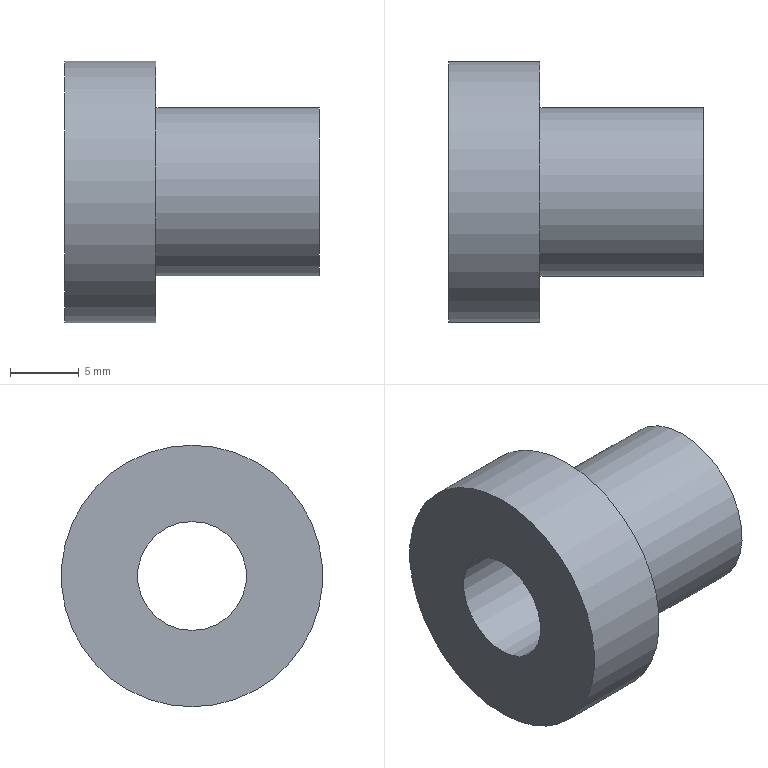Part | NX | features MG0318 steering bushings 2 | 1 solid | 6 faces | box 18.574 x 19.05 x 19.05 mm | volume 2395 mm3 | plane 3 | cylinder 3 | commonest cylinder face diameters 7.938 x1 12.3 x1 19.05 x1
STEP:
#1=CARTESIAN_POINT('',(14.287,0.,3.969));
#2=VERTEX_POINT('',#1);
#3=CARTESIAN_POINT('',(14.287,0.,0.));
#4=DIRECTION('',(-1.,0.,0.));
#5=DIRECTION('',(0.,0.,1.));
#6=AXIS2_PLACEMENT_3D('',#3,#4,#5);
#7=CIRCLE('',#6,3.969);
#8=EDGE_CURVE('',#2,#2,#7,.T.);
#9=ORIENTED_EDGE('',*,*,#8,.F.);
#10=EDGE_LOOP('',(#9));
#11=FACE_BOUND('',#10,.T.);
#12=CARTESIAN_POINT('',(14.287,0.,9.525));
#13=VERTEX_POINT('',#12);
#14=CARTESIAN_POINT('',(14.287,0.,0.));
#15=DIRECTION('',(-1.,0.,0.));
#16=DIRECTION('',(0.,0.,1.));
#17=AXIS2_PLACEMENT_3D('',#14,#15,#16);
#18=CIRCLE('',#17,9.525);
#19=EDGE_CURVE('',#13,#13,#18,.T.);
#20=ORIENTED_EDGE('',*,*,#19,.T.);
#21=EDGE_LOOP('',(#20));
#22=FACE_BOUND('',#21,.T.);
#23=CARTESIAN_POINT('',(14.287,3.969,0.));
#24=DIRECTION('',(1.,0.,0.));
#25=DIRECTION('',(0.,0.,-1.));
#26=AXIS2_PLACEMENT_3D('',#23,#24,#25);
#27=PLANE('',#26);
#28=ADVANCED_FACE('',(#11,#22),#27,.F.);
#29=ORIENTED_EDGE('',*,*,#19,.F.);
#30=EDGE_LOOP('',(#29));
#31=FACE_BOUND('',#30,.T.);
#32=CARTESIAN_POINT('',(20.951,0.,9.525));
#33=VERTEX_POINT('',#32);
#34=CARTESIAN_POINT('',(20.951,0.,0.));
#35=DIRECTION('',(-1.,0.,0.));
#36=DIRECTION('',(0.,0.,1.));
#37=AXIS2_PLACEMENT_3D('',#34,#35,#36);
#38=CIRCLE('',#37,9.525);
#39=EDGE_CURVE('',#33,#33,#38,.T.);
#40=ORIENTED_EDGE('',*,*,#39,.T.);
#41=EDGE_LOOP('',(#40));
#42=FACE_BOUND('',#41,.T.);
#43=CARTESIAN_POINT('',(0.,0.,0.));
#44=DIRECTION('',(-1.,0.,0.));
#45=DIRECTION('',(0.,0.,1.));
#46=AXIS2_PLACEMENT_3D('',#43,#44,#45);
#47=CYLINDRICAL_SURFACE('',#46,9.525);
#48=ADVANCED_FACE('',(#31,#42),#47,.T.);
#49=ORIENTED_EDGE('',*,*,#39,.F.);
#50=EDGE_LOOP('',(#49));
#51=FACE_BOUND('',#50,.T.);
#52=CARTESIAN_POINT('',(20.951,0.,6.15));
#53=VERTEX_POINT('',#52);
#54=CARTESIAN_POINT('',(20.951,0.,0.));
#55=DIRECTION('',(-1.,0.,0.));
#56=DIRECTION('',(0.,0.,1.));
#57=AXIS2_PLACEMENT_3D('',#54,#55,#56);
#58=CIRCLE('',#57,6.15);
#59=EDGE_CURVE('',#53,#53,#58,.T.);
#60=ORIENTED_EDGE('',*,*,#59,.T.);
#61=EDGE_LOOP('',(#60));
#62=FACE_BOUND('',#61,.T.);
#63=CARTESIAN_POINT('',(20.951,6.35,0.));
#64=DIRECTION('',(-1.,0.,0.));
#65=DIRECTION('',(0.,0.,1.));
#66=AXIS2_PLACEMENT_3D('',#63,#64,#65);
#67=PLANE('',#66);
#68=ADVANCED_FACE('',(#51,#62),#67,.F.);
#69=ORIENTED_EDGE('',*,*,#59,.F.);
#70=EDGE_LOOP('',(#69));
#71=FACE_BOUND('',#70,.T.);
#72=CARTESIAN_POINT('',(32.861,0.,6.15));
#73=VERTEX_POINT('',#72);
#74=CARTESIAN_POINT('',(32.861,0.,0.));
#75=DIRECTION('',(-1.,0.,0.));
#76=DIRECTION('',(0.,0.,1.));
#77=AXIS2_PLACEMENT_3D('',#74,#75,#76);
#78=CIRCLE('',#77,6.15);
#79=EDGE_CURVE('',#73,#73,#78,.T.);
#80=ORIENTED_EDGE('',*,*,#79,.T.);
#81=EDGE_LOOP('',(#80));
#82=FACE_BOUND('',#81,.T.);
#83=CARTESIAN_POINT('',(0.,0.,0.));
#84=DIRECTION('',(-1.,0.,0.));
#85=DIRECTION('',(0.,0.,1.));
#86=AXIS2_PLACEMENT_3D('',#83,#84,#85);
#87=CYLINDRICAL_SURFACE('',#86,6.15);
#88=ADVANCED_FACE('',(#71,#82),#87,.T.);
#89=ORIENTED_EDGE('',*,*,#79,.F.);
#90=EDGE_LOOP('',(#89));
#91=FACE_BOUND('',#90,.T.);
#92=CARTESIAN_POINT('',(32.861,0.,3.969));
#93=VERTEX_POINT('',#92);
#94=CARTESIAN_POINT('',(32.861,0.,0.));
#95=DIRECTION('',(-1.,0.,0.));
#96=DIRECTION('',(0.,0.,1.));
#97=AXIS2_PLACEMENT_3D('',#94,#95,#96);
#98=CIRCLE('',#97,3.969);
#99=EDGE_CURVE('',#93,#93,#98,.T.);
#100=ORIENTED_EDGE('',*,*,#99,.T.);
#101=EDGE_LOOP('',(#100));
#102=FACE_BOUND('',#101,.T.);
#103=CARTESIAN_POINT('',(32.861,3.969,0.));
#104=DIRECTION('',(-1.,0.,0.));
#105=DIRECTION('',(0.,0.,1.));
#106=AXIS2_PLACEMENT_3D('',#103,#104,#105);
#107=PLANE('',#106);
#108=ADVANCED_FACE('',(#91,#102),#107,.F.);
#109=ORIENTED_EDGE('',*,*,#99,.F.);
#110=EDGE_LOOP('',(#109));
#111=FACE_BOUND('',#110,.T.);
#112=ORIENTED_EDGE('',*,*,#8,.T.);
#113=EDGE_LOOP('',(#112));
#114=FACE_BOUND('',#113,.T.);
#115=CARTESIAN_POINT('',(0.,0.,0.));
#116=DIRECTION('',(-1.,0.,0.));
#117=DIRECTION('',(0.,0.,1.));
#118=AXIS2_PLACEMENT_3D('',#115,#116,#117);
#119=CYLINDRICAL_SURFACE('',#118,3.969);
#120=ADVANCED_FACE('',(#111,#114),#119,.F.);
#121=CLOSED_SHELL('',(#28,#48,#68,#88,#108,#120));
#122=MANIFOLD_SOLID_BREP('',#121);
#123=(LENGTH_UNIT()NAMED_UNIT(*)SI_UNIT(.MILLI.,.METRE.));
#124=UNCERTAINTY_MEASURE_WITH_UNIT(LENGTH_MEASURE(0.00001),#123,'','');
#125=(NAMED_UNIT(*)PLANE_ANGLE_UNIT()SI_UNIT($,.RADIAN.));
#126=(NAMED_UNIT(*)SI_UNIT($,.STERADIAN.)SOLID_ANGLE_UNIT());
#127=(GEOMETRIC_REPRESENTATION_CONTEXT(3)GLOBAL_UNCERTAINTY_ASSIGNED_CONTEXT((#124))GLOBAL_UNIT_ASSIGNED_CONTEXT((#123,#125,#126))REPRESENTATION_CONTEXT('',''));
#128=ADVANCED_BREP_SHAPE_REPRESENTATION('',(#122),#127);